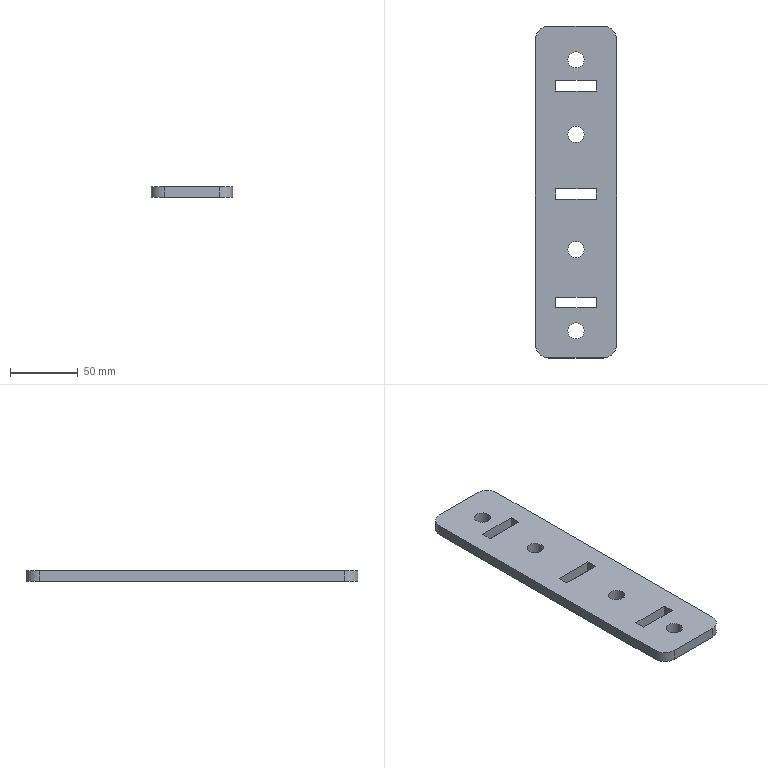Part | SolidWorks | features Fillet 1, FlatPattern 1, SMBaseFlange 1, SheetMetal 1 | 1 solid | 30 faces | box 60 x 245 x 8 mm | volume 107534 mm3 | plane 18 | cylinder 12 | commonest cylinder face diameters 12 x8 20 x4
STEP:
#1=CARTESIAN_POINT('',(-211.919,15.,8.));
#2=VERTEX_POINT('',#1);
#3=CARTESIAN_POINT('',(-199.919,15.,8.));
#4=VERTEX_POINT('',#3);
#5=CARTESIAN_POINT('',(-205.919,15.,8.));
#6=DIRECTION('',(0.,0.,1.));
#7=DIRECTION('',(1.,0.,0.));
#8=AXIS2_PLACEMENT_3D('',#5,#6,#7);
#9=CIRCLE('',#8,6.);
#10=EDGE_CURVE('',#2,#4,#9,.T.);
#11=ORIENTED_EDGE('',*,*,#10,.T.);
#12=CARTESIAN_POINT('',(-199.919,15.,0.));
#13=VERTEX_POINT('',#12);
#14=CARTESIAN_POINT('',(-199.919,15.,8.));
#15=DIRECTION('',(0.,0.,-1.));
#16=VECTOR('',#15,1000.);
#17=LINE('',#14,#16);
#18=EDGE_CURVE('',#4,#13,#17,.T.);
#19=ORIENTED_EDGE('',*,*,#18,.T.);
#20=CARTESIAN_POINT('',(-211.919,15.,0.));
#21=VERTEX_POINT('',#20);
#22=CARTESIAN_POINT('',(-205.919,15.,0.));
#23=DIRECTION('',(0.,0.,1.));
#24=DIRECTION('',(1.,0.,0.));
#25=AXIS2_PLACEMENT_3D('',#22,#23,#24);
#26=CIRCLE('',#25,6.);
#27=EDGE_CURVE('',#21,#13,#26,.T.);
#28=ORIENTED_EDGE('',*,*,#27,.F.);
#29=CARTESIAN_POINT('',(-211.919,15.,8.));
#30=DIRECTION('',(0.,0.,-1.));
#31=VECTOR('',#30,1000.);
#32=LINE('',#29,#31);
#33=EDGE_CURVE('',#2,#21,#32,.T.);
#34=ORIENTED_EDGE('',*,*,#33,.F.);
#35=EDGE_LOOP('',(#11,#19,#28,#34));
#36=FACE_OUTER_BOUND('',#35,.T.);
#37=CARTESIAN_POINT('',(-205.919,15.,8.));
#38=DIRECTION('',(0.,0.,-1.));
#39=DIRECTION('',(-1.,0.,0.));
#40=AXIS2_PLACEMENT_3D('',#37,#38,#39);
#41=CYLINDRICAL_SURFACE('',#40,6.);
#42=ADVANCED_FACE('',(#36),#41,.F.);
#43=CARTESIAN_POINT('',(-211.919,-185.,8.));
#44=VERTEX_POINT('',#43);
#45=CARTESIAN_POINT('',(-199.919,-185.,8.));
#46=VERTEX_POINT('',#45);
#47=CARTESIAN_POINT('',(-205.919,-185.,8.));
#48=DIRECTION('',(0.,0.,1.));
#49=DIRECTION('',(1.,0.,0.));
#50=AXIS2_PLACEMENT_3D('',#47,#48,#49);
#51=CIRCLE('',#50,6.);
#52=EDGE_CURVE('',#44,#46,#51,.T.);
#53=ORIENTED_EDGE('',*,*,#52,.T.);
#54=CARTESIAN_POINT('',(-199.919,-185.,0.));
#55=VERTEX_POINT('',#54);
#56=CARTESIAN_POINT('',(-199.919,-185.,8.));
#57=DIRECTION('',(0.,0.,-1.));
#58=VECTOR('',#57,1000.);
#59=LINE('',#56,#58);
#60=EDGE_CURVE('',#46,#55,#59,.T.);
#61=ORIENTED_EDGE('',*,*,#60,.T.);
#62=CARTESIAN_POINT('',(-211.919,-185.,0.));
#63=VERTEX_POINT('',#62);
#64=CARTESIAN_POINT('',(-205.919,-185.,0.));
#65=DIRECTION('',(0.,0.,1.));
#66=DIRECTION('',(1.,0.,0.));
#67=AXIS2_PLACEMENT_3D('',#64,#65,#66);
#68=CIRCLE('',#67,6.);
#69=EDGE_CURVE('',#63,#55,#68,.T.);
#70=ORIENTED_EDGE('',*,*,#69,.F.);
#71=CARTESIAN_POINT('',(-211.919,-185.,8.));
#72=DIRECTION('',(0.,0.,-1.));
#73=VECTOR('',#72,1000.);
#74=LINE('',#71,#73);
#75=EDGE_CURVE('',#44,#63,#74,.T.);
#76=ORIENTED_EDGE('',*,*,#75,.F.);
#77=EDGE_LOOP('',(#53,#61,#70,#76));
#78=FACE_OUTER_BOUND('',#77,.T.);
#79=CARTESIAN_POINT('',(-205.919,-185.,8.));
#80=DIRECTION('',(0.,0.,-1.));
#81=DIRECTION('',(-1.,0.,0.));
#82=AXIS2_PLACEMENT_3D('',#79,#80,#81);
#83=CYLINDRICAL_SURFACE('',#82,6.);
#84=ADVANCED_FACE('',(#78),#83,.F.);
#85=CARTESIAN_POINT('',(-211.919,-125.,8.));
#86=VERTEX_POINT('',#85);
#87=CARTESIAN_POINT('',(-199.919,-125.,8.));
#88=VERTEX_POINT('',#87);
#89=CARTESIAN_POINT('',(-205.919,-125.,8.));
#90=DIRECTION('',(0.,0.,1.));
#91=DIRECTION('',(1.,0.,0.));
#92=AXIS2_PLACEMENT_3D('',#89,#90,#91);
#93=CIRCLE('',#92,6.);
#94=EDGE_CURVE('',#86,#88,#93,.T.);
#95=ORIENTED_EDGE('',*,*,#94,.T.);
#96=CARTESIAN_POINT('',(-199.919,-125.,0.));
#97=VERTEX_POINT('',#96);
#98=CARTESIAN_POINT('',(-199.919,-125.,8.));
#99=DIRECTION('',(0.,0.,-1.));
#100=VECTOR('',#99,1000.);
#101=LINE('',#98,#100);
#102=EDGE_CURVE('',#88,#97,#101,.T.);
#103=ORIENTED_EDGE('',*,*,#102,.T.);
#104=CARTESIAN_POINT('',(-211.919,-125.,0.));
#105=VERTEX_POINT('',#104);
#106=CARTESIAN_POINT('',(-205.919,-125.,0.));
#107=DIRECTION('',(0.,0.,1.));
#108=DIRECTION('',(1.,0.,0.));
#109=AXIS2_PLACEMENT_3D('',#106,#107,#108);
#110=CIRCLE('',#109,6.);
#111=EDGE_CURVE('',#105,#97,#110,.T.);
#112=ORIENTED_EDGE('',*,*,#111,.F.);
#113=CARTESIAN_POINT('',(-211.919,-125.,8.));
#114=DIRECTION('',(0.,0.,-1.));
#115=VECTOR('',#114,1000.);
#116=LINE('',#113,#115);
#117=EDGE_CURVE('',#86,#105,#116,.T.);
#118=ORIENTED_EDGE('',*,*,#117,.F.);
#119=EDGE_LOOP('',(#95,#103,#112,#118));
#120=FACE_OUTER_BOUND('',#119,.T.);
#121=CARTESIAN_POINT('',(-205.919,-125.,8.));
#122=DIRECTION('',(0.,0.,-1.));
#123=DIRECTION('',(-1.,0.,0.));
#124=AXIS2_PLACEMENT_3D('',#121,#122,#123);
#125=CYLINDRICAL_SURFACE('',#124,6.);
#126=ADVANCED_FACE('',(#120),#125,.F.);
#127=CARTESIAN_POINT('',(-211.919,-40.,8.));
#128=VERTEX_POINT('',#127);
#129=CARTESIAN_POINT('',(-199.919,-40.,8.));
#130=VERTEX_POINT('',#129);
#131=CARTESIAN_POINT('',(-205.919,-40.,8.));
#132=DIRECTION('',(0.,0.,1.));
#133=DIRECTION('',(1.,0.,0.));
#134=AXIS2_PLACEMENT_3D('',#131,#132,#133);
#135=CIRCLE('',#134,6.);
#136=EDGE_CURVE('',#128,#130,#135,.T.);
#137=ORIENTED_EDGE('',*,*,#136,.T.);
#138=CARTESIAN_POINT('',(-199.919,-40.,0.));
#139=VERTEX_POINT('',#138);
#140=CARTESIAN_POINT('',(-199.919,-40.,8.));
#141=DIRECTION('',(0.,0.,-1.));
#142=VECTOR('',#141,1000.);
#143=LINE('',#140,#142);
#144=EDGE_CURVE('',#130,#139,#143,.T.);
#145=ORIENTED_EDGE('',*,*,#144,.T.);
#146=CARTESIAN_POINT('',(-211.919,-40.,0.));
#147=VERTEX_POINT('',#146);
#148=CARTESIAN_POINT('',(-205.919,-40.,0.));
#149=DIRECTION('',(0.,0.,1.));
#150=DIRECTION('',(1.,0.,0.));
#151=AXIS2_PLACEMENT_3D('',#148,#149,#150);
#152=CIRCLE('',#151,6.);
#153=EDGE_CURVE('',#147,#139,#152,.T.);
#154=ORIENTED_EDGE('',*,*,#153,.F.);
#155=CARTESIAN_POINT('',(-211.919,-40.,8.));
#156=DIRECTION('',(0.,0.,-1.));
#157=VECTOR('',#156,1000.);
#158=LINE('',#155,#157);
#159=EDGE_CURVE('',#128,#147,#158,.T.);
#160=ORIENTED_EDGE('',*,*,#159,.F.);
#161=EDGE_LOOP('',(#137,#145,#154,#160));
#162=FACE_OUTER_BOUND('',#161,.T.);
#163=CARTESIAN_POINT('',(-205.919,-40.,8.));
#164=DIRECTION('',(0.,0.,-1.));
#165=DIRECTION('',(-1.,0.,0.));
#166=AXIS2_PLACEMENT_3D('',#163,#164,#165);
#167=CYLINDRICAL_SURFACE('',#166,6.);
#168=ADVANCED_FACE('',(#162),#167,.F.);
#169=ORIENTED_EDGE('',*,*,#52,.F.);
#170=CARTESIAN_POINT('',(-205.919,-185.,8.));
#171=DIRECTION('',(0.,0.,1.));
#172=DIRECTION('',(1.,0.,0.));
#173=AXIS2_PLACEMENT_3D('',#170,#171,#172);
#174=CIRCLE('',#173,6.);
#175=EDGE_CURVE('',#46,#44,#174,.T.);
#176=ORIENTED_EDGE('',*,*,#175,.F.);
#177=EDGE_LOOP('',(#169,#176));
#178=FACE_BOUND('',#177,.T.);
#179=ORIENTED_EDGE('',*,*,#136,.F.);
#180=CARTESIAN_POINT('',(-205.919,-40.,8.));
#181=DIRECTION('',(0.,0.,1.));
#182=DIRECTION('',(1.,0.,0.));
#183=AXIS2_PLACEMENT_3D('',#180,#181,#182);
#184=CIRCLE('',#183,6.);
#185=EDGE_CURVE('',#130,#128,#184,.T.);
#186=ORIENTED_EDGE('',*,*,#185,.F.);
#187=EDGE_LOOP('',(#179,#186));
#188=FACE_BOUND('',#187,.T.);
#189=CARTESIAN_POINT('',(-235.919,30.,8.));
#190=VERTEX_POINT('',#189);
#191=CARTESIAN_POINT('',(-235.919,-195.,8.));
#192=VERTEX_POINT('',#191);
#193=CARTESIAN_POINT('',(-235.919,40.,8.));
#194=DIRECTION('',(0.,-1.,0.));
#195=VECTOR('',#194,1000.);
#196=LINE('',#193,#195);
#197=EDGE_CURVE('',#190,#192,#196,.T.);
#198=ORIENTED_EDGE('',*,*,#197,.T.);
#199=CARTESIAN_POINT('',(-225.919,-205.,8.));
#200=VERTEX_POINT('',#199);
#201=CARTESIAN_POINT('',(-225.919,-195.,8.));
#202=DIRECTION('',(0.,0.,1.));
#203=DIRECTION('',(1.,0.,0.));
#204=AXIS2_PLACEMENT_3D('',#201,#202,#203);
#205=CIRCLE('',#204,10.);
#206=EDGE_CURVE('',#192,#200,#205,.T.);
#207=ORIENTED_EDGE('',*,*,#206,.T.);
#208=CARTESIAN_POINT('',(-185.919,-205.,8.));
#209=VERTEX_POINT('',#208);
#210=CARTESIAN_POINT('',(-235.919,-205.,8.));
#211=DIRECTION('',(1.,0.,0.));
#212=VECTOR('',#211,1000.);
#213=LINE('',#210,#212);
#214=EDGE_CURVE('',#200,#209,#213,.T.);
#215=ORIENTED_EDGE('',*,*,#214,.T.);
#216=CARTESIAN_POINT('',(-175.919,-195.,8.));
#217=VERTEX_POINT('',#216);
#218=CARTESIAN_POINT('',(-185.919,-195.,8.));
#219=DIRECTION('',(0.,0.,1.));
#220=DIRECTION('',(1.,0.,0.));
#221=AXIS2_PLACEMENT_3D('',#218,#219,#220);
#222=CIRCLE('',#221,10.);
#223=EDGE_CURVE('',#209,#217,#222,.T.);
#224=ORIENTED_EDGE('',*,*,#223,.T.);
#225=CARTESIAN_POINT('',(-175.919,30.,8.));
#226=VERTEX_POINT('',#225);
#227=CARTESIAN_POINT('',(-175.919,-205.,8.));
#228=DIRECTION('',(0.,1.,0.));
#229=VECTOR('',#228,1000.);
#230=LINE('',#227,#229);
#231=EDGE_CURVE('',#217,#226,#230,.T.);
#232=ORIENTED_EDGE('',*,*,#231,.T.);
#233=CARTESIAN_POINT('',(-185.919,40.,8.));
#234=VERTEX_POINT('',#233);
#235=CARTESIAN_POINT('',(-185.919,30.,8.));
#236=DIRECTION('',(0.,0.,1.));
#237=DIRECTION('',(1.,0.,0.));
#238=AXIS2_PLACEMENT_3D('',#235,#236,#237);
#239=CIRCLE('',#238,10.);
#240=EDGE_CURVE('',#226,#234,#239,.T.);
#241=ORIENTED_EDGE('',*,*,#240,.T.);
#242=CARTESIAN_POINT('',(-225.919,40.,8.));
#243=VERTEX_POINT('',#242);
#244=CARTESIAN_POINT('',(-175.919,40.,8.));
#245=DIRECTION('',(-1.,0.,0.));
#246=VECTOR('',#245,1000.);
#247=LINE('',#244,#246);
#248=EDGE_CURVE('',#234,#243,#247,.T.);
#249=ORIENTED_EDGE('',*,*,#248,.T.);
#250=CARTESIAN_POINT('',(-225.919,30.,8.));
#251=DIRECTION('',(0.,0.,1.));
#252=DIRECTION('',(1.,0.,0.));
#253=AXIS2_PLACEMENT_3D('',#250,#251,#252);
#254=CIRCLE('',#253,10.);
#255=EDGE_CURVE('',#243,#190,#254,.T.);
#256=ORIENTED_EDGE('',*,*,#255,.T.);
#257=EDGE_LOOP('',(#198,#207,#215,#224,#232,#241,#249,#256));
#258=FACE_OUTER_BOUND('',#257,.T.);
#259=CARTESIAN_POINT('',(-190.919,-160.,8.));
#260=VERTEX_POINT('',#259);
#261=CARTESIAN_POINT('',(-220.919,-160.,8.));
#262=VERTEX_POINT('',#261);
#263=CARTESIAN_POINT('',(-220.919,-160.,8.));
#264=DIRECTION('',(-1.,0.,0.));
#265=VECTOR('',#264,1000.);
#266=LINE('',#263,#265);
#267=EDGE_CURVE('',#260,#262,#266,.T.);
#268=ORIENTED_EDGE('',*,*,#267,.F.);
#269=CARTESIAN_POINT('',(-190.919,-168.,8.));
#270=VERTEX_POINT('',#269);
#271=CARTESIAN_POINT('',(-190.919,-160.,8.));
#272=DIRECTION('',(0.,1.,0.));
#273=VECTOR('',#272,1000.);
#274=LINE('',#271,#273);
#275=EDGE_CURVE('',#270,#260,#274,.T.);
#276=ORIENTED_EDGE('',*,*,#275,.F.);
#277=CARTESIAN_POINT('',(-220.919,-168.,8.));
#278=VERTEX_POINT('',#277);
#279=CARTESIAN_POINT('',(-190.919,-168.,8.));
#280=DIRECTION('',(1.,0.,0.));
#281=VECTOR('',#280,1000.);
#282=LINE('',#279,#281);
#283=EDGE_CURVE('',#278,#270,#282,.T.);
#284=ORIENTED_EDGE('',*,*,#283,.F.);
#285=CARTESIAN_POINT('',(-220.919,-168.,8.));
#286=DIRECTION('',(0.,-1.,0.));
#287=VECTOR('',#286,1000.);
#288=LINE('',#285,#287);
#289=EDGE_CURVE('',#262,#278,#288,.T.);
#290=ORIENTED_EDGE('',*,*,#289,.F.);
#291=EDGE_LOOP('',(#268,#276,#284,#290));
#292=FACE_BOUND('',#291,.T.);
#293=CARTESIAN_POINT('',(-190.919,-88.,8.));
#294=VERTEX_POINT('',#293);
#295=CARTESIAN_POINT('',(-190.919,-80.,8.));
#296=VERTEX_POINT('',#295);
#297=CARTESIAN_POINT('',(-190.919,-80.,8.));
#298=DIRECTION('',(0.,1.,0.));
#299=VECTOR('',#298,1000.);
#300=LINE('',#297,#299);
#301=EDGE_CURVE('',#294,#296,#300,.T.);
#302=ORIENTED_EDGE('',*,*,#301,.F.);
#303=CARTESIAN_POINT('',(-220.919,-88.,8.));
#304=VERTEX_POINT('',#303);
#305=CARTESIAN_POINT('',(-190.919,-88.,8.));
#306=DIRECTION('',(1.,0.,0.));
#307=VECTOR('',#306,1000.);
#308=LINE('',#305,#307);
#309=EDGE_CURVE('',#304,#294,#308,.T.);
#310=ORIENTED_EDGE('',*,*,#309,.F.);
#311=CARTESIAN_POINT('',(-220.919,-80.,8.));
#312=VERTEX_POINT('',#311);
#313=CARTESIAN_POINT('',(-220.919,-88.,8.));
#314=DIRECTION('',(0.,-1.,0.));
#315=VECTOR('',#314,1000.);
#316=LINE('',#313,#315);
#317=EDGE_CURVE('',#312,#304,#316,.T.);
#318=ORIENTED_EDGE('',*,*,#317,.F.);
#319=CARTESIAN_POINT('',(-220.919,-80.,8.));
#320=DIRECTION('',(-1.,0.,0.));
#321=VECTOR('',#320,1000.);
#322=LINE('',#319,#321);
#323=EDGE_CURVE('',#296,#312,#322,.T.);
#324=ORIENTED_EDGE('',*,*,#323,.F.);
#325=EDGE_LOOP('',(#302,#310,#318,#324));
#326=FACE_BOUND('',#325,.T.);
#327=CARTESIAN_POINT('',(-190.919,-8.,8.));
#328=VERTEX_POINT('',#327);
#329=CARTESIAN_POINT('',(-190.919,0.,8.));
#330=VERTEX_POINT('',#329);
#331=CARTESIAN_POINT('',(-190.919,0.,8.));
#332=DIRECTION('',(0.,1.,0.));
#333=VECTOR('',#332,1000.);
#334=LINE('',#331,#333);
#335=EDGE_CURVE('',#328,#330,#334,.T.);
#336=ORIENTED_EDGE('',*,*,#335,.F.);
#337=CARTESIAN_POINT('',(-220.919,-8.,8.));
#338=VERTEX_POINT('',#337);
#339=CARTESIAN_POINT('',(-190.919,-8.,8.));
#340=DIRECTION('',(1.,0.,0.));
#341=VECTOR('',#340,1000.);
#342=LINE('',#339,#341);
#343=EDGE_CURVE('',#338,#328,#342,.T.);
#344=ORIENTED_EDGE('',*,*,#343,.F.);
#345=CARTESIAN_POINT('',(-220.919,0.,8.));
#346=VERTEX_POINT('',#345);
#347=CARTESIAN_POINT('',(-220.919,-8.,8.));
#348=DIRECTION('',(0.,-1.,0.));
#349=VECTOR('',#348,1000.);
#350=LINE('',#347,#349);
#351=EDGE_CURVE('',#346,#338,#350,.T.);
#352=ORIENTED_EDGE('',*,*,#351,.F.);
#353=CARTESIAN_POINT('',(-220.919,0.,8.));
#354=DIRECTION('',(-1.,0.,0.));
#355=VECTOR('',#354,1000.);
#356=LINE('',#353,#355);
#357=EDGE_CURVE('',#330,#346,#356,.T.);
#358=ORIENTED_EDGE('',*,*,#357,.F.);
#359=EDGE_LOOP('',(#336,#344,#352,#358));
#360=FACE_BOUND('',#359,.T.);
#361=ORIENTED_EDGE('',*,*,#94,.F.);
#362=CARTESIAN_POINT('',(-205.919,-125.,8.));
#363=DIRECTION('',(0.,0.,1.));
#364=DIRECTION('',(1.,0.,0.));
#365=AXIS2_PLACEMENT_3D('',#362,#363,#364);
#366=CIRCLE('',#365,6.);
#367=EDGE_CURVE('',#88,#86,#366,.T.);
#368=ORIENTED_EDGE('',*,*,#367,.F.);
#369=EDGE_LOOP('',(#361,#368));
#370=FACE_BOUND('',#369,.T.);
#371=ORIENTED_EDGE('',*,*,#10,.F.);
#372=CARTESIAN_POINT('',(-205.919,15.,8.));
#373=DIRECTION('',(0.,0.,1.));
#374=DIRECTION('',(1.,0.,0.));
#375=AXIS2_PLACEMENT_3D('',#372,#373,#374);
#376=CIRCLE('',#375,6.);
#377=EDGE_CURVE('',#4,#2,#376,.T.);
#378=ORIENTED_EDGE('',*,*,#377,.F.);
#379=EDGE_LOOP('',(#371,#378));
#380=FACE_BOUND('',#379,.T.);
#381=CARTESIAN_POINT('',(0.,0.,8.));
#382=DIRECTION('',(0.,0.,1.));
#383=DIRECTION('',(1.,0.,0.));
#384=AXIS2_PLACEMENT_3D('',#381,#382,#383);
#385=PLANE('',#384);
#386=ADVANCED_FACE('',(#178,#188,#258,#292,#326,#360,#370,#380),#385,.T.);
#387=CARTESIAN_POINT('',(-220.919,-88.,0.));
#388=VERTEX_POINT('',#387);
#389=CARTESIAN_POINT('',(-190.919,-88.,0.));
#390=VERTEX_POINT('',#389);
#391=CARTESIAN_POINT('',(-190.919,-88.,0.));
#392=DIRECTION('',(1.,0.,0.));
#393=VECTOR('',#392,1000.);
#394=LINE('',#391,#393);
#395=EDGE_CURVE('',#388,#390,#394,.T.);
#396=ORIENTED_EDGE('',*,*,#395,.T.);
#397=CARTESIAN_POINT('',(-190.919,-80.,0.));
#398=VERTEX_POINT('',#397);
#399=CARTESIAN_POINT('',(-190.919,-80.,0.));
#400=DIRECTION('',(0.,1.,0.));
#401=VECTOR('',#400,1000.);
#402=LINE('',#399,#401);
#403=EDGE_CURVE('',#390,#398,#402,.T.);
#404=ORIENTED_EDGE('',*,*,#403,.T.);
#405=CARTESIAN_POINT('',(-220.919,-80.,0.));
#406=VERTEX_POINT('',#405);
#407=CARTESIAN_POINT('',(-220.919,-80.,0.));
#408=DIRECTION('',(-1.,0.,0.));
#409=VECTOR('',#408,1000.);
#410=LINE('',#407,#409);
#411=EDGE_CURVE('',#398,#406,#410,.T.);
#412=ORIENTED_EDGE('',*,*,#411,.T.);
#413=CARTESIAN_POINT('',(-220.919,-88.,0.));
#414=DIRECTION('',(0.,-1.,0.));
#415=VECTOR('',#414,1000.);
#416=LINE('',#413,#415);
#417=EDGE_CURVE('',#406,#388,#416,.T.);
#418=ORIENTED_EDGE('',*,*,#417,.T.);
#419=EDGE_LOOP('',(#396,#404,#412,#418));
#420=FACE_BOUND('',#419,.T.);
#421=CARTESIAN_POINT('',(-225.919,-205.,0.));
#422=VERTEX_POINT('',#421);
#423=CARTESIAN_POINT('',(-185.919,-205.,0.));
#424=VERTEX_POINT('',#423);
#425=CARTESIAN_POINT('',(-235.919,-205.,0.));
#426=DIRECTION('',(1.,0.,0.));
#427=VECTOR('',#426,1000.);
#428=LINE('',#425,#427);
#429=EDGE_CURVE('',#422,#424,#428,.T.);
#430=ORIENTED_EDGE('',*,*,#429,.F.);
#431=CARTESIAN_POINT('',(-235.919,-195.,0.));
#432=VERTEX_POINT('',#431);
#433=CARTESIAN_POINT('',(-225.919,-195.,0.));
#434=DIRECTION('',(0.,0.,-1.));
#435=DIRECTION('',(1.,0.,0.));
#436=AXIS2_PLACEMENT_3D('',#433,#434,#435);
#437=CIRCLE('',#436,10.);
#438=EDGE_CURVE('',#422,#432,#437,.T.);
#439=ORIENTED_EDGE('',*,*,#438,.T.);
#440=CARTESIAN_POINT('',(-235.919,30.,0.));
#441=VERTEX_POINT('',#440);
#442=CARTESIAN_POINT('',(-235.919,40.,0.));
#443=DIRECTION('',(0.,-1.,0.));
#444=VECTOR('',#443,1000.);
#445=LINE('',#442,#444);
#446=EDGE_CURVE('',#441,#432,#445,.T.);
#447=ORIENTED_EDGE('',*,*,#446,.F.);
#448=CARTESIAN_POINT('',(-225.919,40.,0.));
#449=VERTEX_POINT('',#448);
#450=CARTESIAN_POINT('',(-225.919,30.,0.));
#451=DIRECTION('',(0.,0.,-1.));
#452=DIRECTION('',(1.,0.,0.));
#453=AXIS2_PLACEMENT_3D('',#450,#451,#452);
#454=CIRCLE('',#453,10.);
#455=EDGE_CURVE('',#441,#449,#454,.T.);
#456=ORIENTED_EDGE('',*,*,#455,.T.);
#457=CARTESIAN_POINT('',(-185.919,40.,0.));
#458=VERTEX_POINT('',#457);
#459=CARTESIAN_POINT('',(-175.919,40.,0.));
#460=DIRECTION('',(-1.,0.,0.));
#461=VECTOR('',#460,1000.);
#462=LINE('',#459,#461);
#463=EDGE_CURVE('',#458,#449,#462,.T.);
#464=ORIENTED_EDGE('',*,*,#463,.F.);
#465=CARTESIAN_POINT('',(-175.919,30.,0.));
#466=VERTEX_POINT('',#465);
#467=CARTESIAN_POINT('',(-185.919,30.,0.));
#468=DIRECTION('',(0.,0.,-1.));
#469=DIRECTION('',(1.,0.,0.));
#470=AXIS2_PLACEMENT_3D('',#467,#468,#469);
#471=CIRCLE('',#470,10.);
#472=EDGE_CURVE('',#458,#466,#471,.T.);
#473=ORIENTED_EDGE('',*,*,#472,.T.);
#474=CARTESIAN_POINT('',(-175.919,-195.,0.));
#475=VERTEX_POINT('',#474);
#476=CARTESIAN_POINT('',(-175.919,-205.,0.));
#477=DIRECTION('',(0.,1.,0.));
#478=VECTOR('',#477,1000.);
#479=LINE('',#476,#478);
#480=EDGE_CURVE('',#475,#466,#479,.T.);
#481=ORIENTED_EDGE('',*,*,#480,.F.);
#482=CARTESIAN_POINT('',(-185.919,-195.,0.));
#483=DIRECTION('',(0.,0.,-1.));
#484=DIRECTION('',(1.,0.,0.));
#485=AXIS2_PLACEMENT_3D('',#482,#483,#484);
#486=CIRCLE('',#485,10.);
#487=EDGE_CURVE('',#475,#424,#486,.T.);
#488=ORIENTED_EDGE('',*,*,#487,.T.);
#489=EDGE_LOOP('',(#430,#439,#447,#456,#464,#473,#481,#488));
#490=FACE_OUTER_BOUND('',#489,.T.);
#491=CARTESIAN_POINT('',(-190.919,-168.,0.));
#492=VERTEX_POINT('',#491);
#493=CARTESIAN_POINT('',(-190.919,-160.,0.));
#494=VERTEX_POINT('',#493);
#495=CARTESIAN_POINT('',(-190.919,-160.,0.));
#496=DIRECTION('',(0.,1.,0.));
#497=VECTOR('',#496,1000.);
#498=LINE('',#495,#497);
#499=EDGE_CURVE('',#492,#494,#498,.T.);
#500=ORIENTED_EDGE('',*,*,#499,.T.);
#501=CARTESIAN_POINT('',(-220.919,-160.,0.));
#502=VERTEX_POINT('',#501);
#503=CARTESIAN_POINT('',(-220.919,-160.,0.));
#504=DIRECTION('',(-1.,0.,0.));
#505=VECTOR('',#504,1000.);
#506=LINE('',#503,#505);
#507=EDGE_CURVE('',#494,#502,#506,.T.);
#508=ORIENTED_EDGE('',*,*,#507,.T.);
#509=CARTESIAN_POINT('',(-220.919,-168.,0.));
#510=VERTEX_POINT('',#509);
#511=CARTESIAN_POINT('',(-220.919,-168.,0.));
#512=DIRECTION('',(0.,-1.,0.));
#513=VECTOR('',#512,1000.);
#514=LINE('',#511,#513);
#515=EDGE_CURVE('',#502,#510,#514,.T.);
#516=ORIENTED_EDGE('',*,*,#515,.T.);
#517=CARTESIAN_POINT('',(-190.919,-168.,0.));
#518=DIRECTION('',(1.,0.,0.));
#519=VECTOR('',#518,1000.);
#520=LINE('',#517,#519);
#521=EDGE_CURVE('',#510,#492,#520,.T.);
#522=ORIENTED_EDGE('',*,*,#521,.T.);
#523=EDGE_LOOP('',(#500,#508,#516,#522));
#524=FACE_BOUND('',#523,.T.);
#525=CARTESIAN_POINT('',(-220.919,-8.,0.));
#526=VERTEX_POINT('',#525);
#527=CARTESIAN_POINT('',(-190.919,-8.,0.));
#528=VERTEX_POINT('',#527);
#529=CARTESIAN_POINT('',(-190.919,-8.,0.));
#530=DIRECTION('',(1.,0.,0.));
#531=VECTOR('',#530,1000.);
#532=LINE('',#529,#531);
#533=EDGE_CURVE('',#526,#528,#532,.T.);
#534=ORIENTED_EDGE('',*,*,#533,.T.);
#535=CARTESIAN_POINT('',(-190.919,0.,0.));
#536=VERTEX_POINT('',#535);
#537=CARTESIAN_POINT('',(-190.919,0.,0.));
#538=DIRECTION('',(0.,1.,0.));
#539=VECTOR('',#538,1000.);
#540=LINE('',#537,#539);
#541=EDGE_CURVE('',#528,#536,#540,.T.);
#542=ORIENTED_EDGE('',*,*,#541,.T.);
#543=CARTESIAN_POINT('',(-220.919,0.,0.));
#544=VERTEX_POINT('',#543);
#545=CARTESIAN_POINT('',(-220.919,0.,0.));
#546=DIRECTION('',(-1.,0.,0.));
#547=VECTOR('',#546,1000.);
#548=LINE('',#545,#547);
#549=EDGE_CURVE('',#536,#544,#548,.T.);
#550=ORIENTED_EDGE('',*,*,#549,.T.);
#551=CARTESIAN_POINT('',(-220.919,-8.,0.));
#552=DIRECTION('',(0.,-1.,0.));
#553=VECTOR('',#552,1000.);
#554=LINE('',#551,#553);
#555=EDGE_CURVE('',#544,#526,#554,.T.);
#556=ORIENTED_EDGE('',*,*,#555,.T.);
#557=EDGE_LOOP('',(#534,#542,#550,#556));
#558=FACE_BOUND('',#557,.T.);
#559=ORIENTED_EDGE('',*,*,#153,.T.);
#560=CARTESIAN_POINT('',(-205.919,-40.,0.));
#561=DIRECTION('',(0.,0.,1.));
#562=DIRECTION('',(1.,0.,0.));
#563=AXIS2_PLACEMENT_3D('',#560,#561,#562);
#564=CIRCLE('',#563,6.);
#565=EDGE_CURVE('',#139,#147,#564,.T.);
#566=ORIENTED_EDGE('',*,*,#565,.T.);
#567=EDGE_LOOP('',(#559,#566));
#568=FACE_BOUND('',#567,.T.);
#569=ORIENTED_EDGE('',*,*,#111,.T.);
#570=CARTESIAN_POINT('',(-205.919,-125.,0.));
#571=DIRECTION('',(0.,0.,1.));
#572=DIRECTION('',(1.,0.,0.));
#573=AXIS2_PLACEMENT_3D('',#570,#571,#572);
#574=CIRCLE('',#573,6.);
#575=EDGE_CURVE('',#97,#105,#574,.T.);
#576=ORIENTED_EDGE('',*,*,#575,.T.);
#577=EDGE_LOOP('',(#569,#576));
#578=FACE_BOUND('',#577,.T.);
#579=ORIENTED_EDGE('',*,*,#69,.T.);
#580=CARTESIAN_POINT('',(-205.919,-185.,0.));
#581=DIRECTION('',(0.,0.,1.));
#582=DIRECTION('',(1.,0.,0.));
#583=AXIS2_PLACEMENT_3D('',#580,#581,#582);
#584=CIRCLE('',#583,6.);
#585=EDGE_CURVE('',#55,#63,#584,.T.);
#586=ORIENTED_EDGE('',*,*,#585,.T.);
#587=EDGE_LOOP('',(#579,#586));
#588=FACE_BOUND('',#587,.T.);
#589=ORIENTED_EDGE('',*,*,#27,.T.);
#590=CARTESIAN_POINT('',(-205.919,15.,0.));
#591=DIRECTION('',(0.,0.,1.));
#592=DIRECTION('',(1.,0.,0.));
#593=AXIS2_PLACEMENT_3D('',#590,#591,#592);
#594=CIRCLE('',#593,6.);
#595=EDGE_CURVE('',#13,#21,#594,.T.);
#596=ORIENTED_EDGE('',*,*,#595,.T.);
#597=EDGE_LOOP('',(#589,#596));
#598=FACE_BOUND('',#597,.T.);
#599=CARTESIAN_POINT('',(0.,0.,0.));
#600=DIRECTION('',(0.,0.,1.));
#601=DIRECTION('',(1.,0.,0.));
#602=AXIS2_PLACEMENT_3D('',#599,#600,#601);
#603=PLANE('',#602);
#604=ADVANCED_FACE('',(#420,#490,#524,#558,#568,#578,#588,#598),#603,.F.);
#605=ORIENTED_EDGE('',*,*,#446,.T.);
#606=CARTESIAN_POINT('',(-235.919,-195.,8.));
#607=DIRECTION('',(0.,0.,1.));
#608=VECTOR('',#607,1000.);
#609=LINE('',#606,#608);
#610=EDGE_CURVE('',#432,#192,#609,.T.);
#611=ORIENTED_EDGE('',*,*,#610,.T.);
#612=ORIENTED_EDGE('',*,*,#197,.F.);
#613=CARTESIAN_POINT('',(-235.919,30.,8.));
#614=DIRECTION('',(0.,0.,-1.));
#615=VECTOR('',#614,1000.);
#616=LINE('',#613,#615);
#617=EDGE_CURVE('',#190,#441,#616,.T.);
#618=ORIENTED_EDGE('',*,*,#617,.T.);
#619=EDGE_LOOP('',(#605,#611,#612,#618));
#620=FACE_OUTER_BOUND('',#619,.T.);
#621=CARTESIAN_POINT('',(-235.919,40.,8.));
#622=DIRECTION('',(1.,0.,0.));
#623=DIRECTION('',(0.,1.,0.));
#624=AXIS2_PLACEMENT_3D('',#621,#622,#623);
#625=PLANE('',#624);
#626=ADVANCED_FACE('',(#620),#625,.F.);
#627=ORIENTED_EDGE('',*,*,#214,.F.);
#628=CARTESIAN_POINT('',(-225.919,-205.,8.));
#629=DIRECTION('',(0.,0.,-1.));
#630=VECTOR('',#629,1000.);
#631=LINE('',#628,#630);
#632=EDGE_CURVE('',#200,#422,#631,.T.);
#633=ORIENTED_EDGE('',*,*,#632,.T.);
#634=ORIENTED_EDGE('',*,*,#429,.T.);
#635=CARTESIAN_POINT('',(-185.919,-205.,8.));
#636=DIRECTION('',(0.,0.,1.));
#637=VECTOR('',#636,1000.);
#638=LINE('',#635,#637);
#639=EDGE_CURVE('',#424,#209,#638,.T.);
#640=ORIENTED_EDGE('',*,*,#639,.T.);
#641=EDGE_LOOP('',(#627,#633,#634,#640));
#642=FACE_OUTER_BOUND('',#641,.T.);
#643=CARTESIAN_POINT('',(-235.919,-205.,8.));
#644=DIRECTION('',(0.,1.,0.));
#645=DIRECTION('',(0.,0.,1.));
#646=AXIS2_PLACEMENT_3D('',#643,#644,#645);
#647=PLANE('',#646);
#648=ADVANCED_FACE('',(#642),#647,.F.);
#649=ORIENTED_EDGE('',*,*,#231,.F.);
#650=CARTESIAN_POINT('',(-175.919,-195.,8.));
#651=DIRECTION('',(0.,0.,-1.));
#652=VECTOR('',#651,1000.);
#653=LINE('',#650,#652);
#654=EDGE_CURVE('',#217,#475,#653,.T.);
#655=ORIENTED_EDGE('',*,*,#654,.T.);
#656=ORIENTED_EDGE('',*,*,#480,.T.);
#657=CARTESIAN_POINT('',(-175.919,30.,8.));
#658=DIRECTION('',(0.,0.,1.));
#659=VECTOR('',#658,1000.);
#660=LINE('',#657,#659);
#661=EDGE_CURVE('',#466,#226,#660,.T.);
#662=ORIENTED_EDGE('',*,*,#661,.T.);
#663=EDGE_LOOP('',(#649,#655,#656,#662));
#664=FACE_OUTER_BOUND('',#663,.T.);
#665=CARTESIAN_POINT('',(-175.919,-205.,8.));
#666=DIRECTION('',(-1.,0.,0.));
#667=DIRECTION('',(0.,0.,1.));
#668=AXIS2_PLACEMENT_3D('',#665,#666,#667);
#669=PLANE('',#668);
#670=ADVANCED_FACE('',(#664),#669,.F.);
#671=ORIENTED_EDGE('',*,*,#248,.F.);
#672=CARTESIAN_POINT('',(-185.919,40.,8.));
#673=DIRECTION('',(0.,0.,-1.));
#674=VECTOR('',#673,1000.);
#675=LINE('',#672,#674);
#676=EDGE_CURVE('',#234,#458,#675,.T.);
#677=ORIENTED_EDGE('',*,*,#676,.T.);
#678=ORIENTED_EDGE('',*,*,#463,.T.);
#679=CARTESIAN_POINT('',(-225.919,40.,8.));
#680=DIRECTION('',(0.,0.,1.));
#681=VECTOR('',#680,1000.);
#682=LINE('',#679,#681);
#683=EDGE_CURVE('',#449,#243,#682,.T.);
#684=ORIENTED_EDGE('',*,*,#683,.T.);
#685=EDGE_LOOP('',(#671,#677,#678,#684));
#686=FACE_OUTER_BOUND('',#685,.T.);
#687=CARTESIAN_POINT('',(-175.919,40.,8.));
#688=DIRECTION('',(0.,-1.,0.));
#689=DIRECTION('',(1.,0.,0.));
#690=AXIS2_PLACEMENT_3D('',#687,#688,#689);
#691=PLANE('',#690);
#692=ADVANCED_FACE('',(#686),#691,.F.);
#693=ORIENTED_EDGE('',*,*,#499,.F.);
#694=CARTESIAN_POINT('',(-190.919,-168.,8.));
#695=DIRECTION('',(0.,0.,-1.));
#696=VECTOR('',#695,1000.);
#697=LINE('',#694,#696);
#698=EDGE_CURVE('',#270,#492,#697,.T.);
#699=ORIENTED_EDGE('',*,*,#698,.F.);
#700=ORIENTED_EDGE('',*,*,#275,.T.);
#701=CARTESIAN_POINT('',(-190.919,-160.,8.));
#702=DIRECTION('',(0.,0.,-1.));
#703=VECTOR('',#702,1000.);
#704=LINE('',#701,#703);
#705=EDGE_CURVE('',#260,#494,#704,.T.);
#706=ORIENTED_EDGE('',*,*,#705,.T.);
#707=EDGE_LOOP('',(#693,#699,#700,#706));
#708=FACE_OUTER_BOUND('',#707,.T.);
#709=CARTESIAN_POINT('',(-190.919,-160.,8.));
#710=DIRECTION('',(-1.,0.,0.));
#711=DIRECTION('',(0.,0.,1.));
#712=AXIS2_PLACEMENT_3D('',#709,#710,#711);
#713=PLANE('',#712);
#714=ADVANCED_FACE('',(#708),#713,.T.);
#715=ORIENTED_EDGE('',*,*,#507,.F.);
#716=ORIENTED_EDGE('',*,*,#705,.F.);
#717=ORIENTED_EDGE('',*,*,#267,.T.);
#718=CARTESIAN_POINT('',(-220.919,-160.,8.));
#719=DIRECTION('',(0.,0.,-1.));
#720=VECTOR('',#719,1000.);
#721=LINE('',#718,#720);
#722=EDGE_CURVE('',#262,#502,#721,.T.);
#723=ORIENTED_EDGE('',*,*,#722,.T.);
#724=EDGE_LOOP('',(#715,#716,#717,#723));
#725=FACE_OUTER_BOUND('',#724,.T.);
#726=CARTESIAN_POINT('',(-220.919,-160.,8.));
#727=DIRECTION('',(0.,-1.,0.));
#728=DIRECTION('',(0.,0.,-1.));
#729=AXIS2_PLACEMENT_3D('',#726,#727,#728);
#730=PLANE('',#729);
#731=ADVANCED_FACE('',(#725),#730,.T.);
#732=ORIENTED_EDGE('',*,*,#515,.F.);
#733=ORIENTED_EDGE('',*,*,#722,.F.);
#734=ORIENTED_EDGE('',*,*,#289,.T.);
#735=CARTESIAN_POINT('',(-220.919,-168.,8.));
#736=DIRECTION('',(0.,0.,-1.));
#737=VECTOR('',#736,1000.);
#738=LINE('',#735,#737);
#739=EDGE_CURVE('',#278,#510,#738,.T.);
#740=ORIENTED_EDGE('',*,*,#739,.T.);
#741=EDGE_LOOP('',(#732,#733,#734,#740));
#742=FACE_OUTER_BOUND('',#741,.T.);
#743=CARTESIAN_POINT('',(-220.919,-168.,8.));
#744=DIRECTION('',(1.,0.,0.));
#745=DIRECTION('',(0.,0.,-1.));
#746=AXIS2_PLACEMENT_3D('',#743,#744,#745);
#747=PLANE('',#746);
#748=ADVANCED_FACE('',(#742),#747,.T.);
#749=ORIENTED_EDGE('',*,*,#521,.F.);
#750=ORIENTED_EDGE('',*,*,#739,.F.);
#751=ORIENTED_EDGE('',*,*,#283,.T.);
#752=ORIENTED_EDGE('',*,*,#698,.T.);
#753=EDGE_LOOP('',(#749,#750,#751,#752));
#754=FACE_OUTER_BOUND('',#753,.T.);
#755=CARTESIAN_POINT('',(-190.919,-168.,8.));
#756=DIRECTION('',(0.,1.,0.));
#757=DIRECTION('',(0.,0.,1.));
#758=AXIS2_PLACEMENT_3D('',#755,#756,#757);
#759=PLANE('',#758);
#760=ADVANCED_FACE('',(#754),#759,.T.);
#761=ORIENTED_EDGE('',*,*,#395,.F.);
#762=CARTESIAN_POINT('',(-220.919,-88.,8.));
#763=DIRECTION('',(0.,0.,-1.));
#764=VECTOR('',#763,1000.);
#765=LINE('',#762,#764);
#766=EDGE_CURVE('',#304,#388,#765,.T.);
#767=ORIENTED_EDGE('',*,*,#766,.F.);
#768=ORIENTED_EDGE('',*,*,#309,.T.);
#769=CARTESIAN_POINT('',(-190.919,-88.,8.));
#770=DIRECTION('',(0.,0.,-1.));
#771=VECTOR('',#770,1000.);
#772=LINE('',#769,#771);
#773=EDGE_CURVE('',#294,#390,#772,.T.);
#774=ORIENTED_EDGE('',*,*,#773,.T.);
#775=EDGE_LOOP('',(#761,#767,#768,#774));
#776=FACE_OUTER_BOUND('',#775,.T.);
#777=CARTESIAN_POINT('',(-190.919,-88.,8.));
#778=DIRECTION('',(0.,1.,0.));
#779=DIRECTION('',(0.,0.,1.));
#780=AXIS2_PLACEMENT_3D('',#777,#778,#779);
#781=PLANE('',#780);
#782=ADVANCED_FACE('',(#776),#781,.T.);
#783=ORIENTED_EDGE('',*,*,#403,.F.);
#784=ORIENTED_EDGE('',*,*,#773,.F.);
#785=ORIENTED_EDGE('',*,*,#301,.T.);
#786=CARTESIAN_POINT('',(-190.919,-80.,8.));
#787=DIRECTION('',(0.,0.,-1.));
#788=VECTOR('',#787,1000.);
#789=LINE('',#786,#788);
#790=EDGE_CURVE('',#296,#398,#789,.T.);
#791=ORIENTED_EDGE('',*,*,#790,.T.);
#792=EDGE_LOOP('',(#783,#784,#785,#791));
#793=FACE_OUTER_BOUND('',#792,.T.);
#794=CARTESIAN_POINT('',(-190.919,-80.,8.));
#795=DIRECTION('',(-1.,0.,0.));
#796=DIRECTION('',(0.,0.,1.));
#797=AXIS2_PLACEMENT_3D('',#794,#795,#796);
#798=PLANE('',#797);
#799=ADVANCED_FACE('',(#793),#798,.T.);
#800=ORIENTED_EDGE('',*,*,#411,.F.);
#801=ORIENTED_EDGE('',*,*,#790,.F.);
#802=ORIENTED_EDGE('',*,*,#323,.T.);
#803=CARTESIAN_POINT('',(-220.919,-80.,8.));
#804=DIRECTION('',(0.,0.,-1.));
#805=VECTOR('',#804,1000.);
#806=LINE('',#803,#805);
#807=EDGE_CURVE('',#312,#406,#806,.T.);
#808=ORIENTED_EDGE('',*,*,#807,.T.);
#809=EDGE_LOOP('',(#800,#801,#802,#808));
#810=FACE_OUTER_BOUND('',#809,.T.);
#811=CARTESIAN_POINT('',(-220.919,-80.,8.));
#812=DIRECTION('',(0.,-1.,0.));
#813=DIRECTION('',(0.,0.,-1.));
#814=AXIS2_PLACEMENT_3D('',#811,#812,#813);
#815=PLANE('',#814);
#816=ADVANCED_FACE('',(#810),#815,.T.);
#817=ORIENTED_EDGE('',*,*,#417,.F.);
#818=ORIENTED_EDGE('',*,*,#807,.F.);
#819=ORIENTED_EDGE('',*,*,#317,.T.);
#820=ORIENTED_EDGE('',*,*,#766,.T.);
#821=EDGE_LOOP('',(#817,#818,#819,#820));
#822=FACE_OUTER_BOUND('',#821,.T.);
#823=CARTESIAN_POINT('',(-220.919,-88.,8.));
#824=DIRECTION('',(1.,0.,0.));
#825=DIRECTION('',(0.,0.,-1.));
#826=AXIS2_PLACEMENT_3D('',#823,#824,#825);
#827=PLANE('',#826);
#828=ADVANCED_FACE('',(#822),#827,.T.);
#829=ORIENTED_EDGE('',*,*,#533,.F.);
#830=CARTESIAN_POINT('',(-220.919,-8.,8.));
#831=DIRECTION('',(0.,0.,-1.));
#832=VECTOR('',#831,1000.);
#833=LINE('',#830,#832);
#834=EDGE_CURVE('',#338,#526,#833,.T.);
#835=ORIENTED_EDGE('',*,*,#834,.F.);
#836=ORIENTED_EDGE('',*,*,#343,.T.);
#837=CARTESIAN_POINT('',(-190.919,-8.,8.));
#838=DIRECTION('',(0.,0.,-1.));
#839=VECTOR('',#838,1000.);
#840=LINE('',#837,#839);
#841=EDGE_CURVE('',#328,#528,#840,.T.);
#842=ORIENTED_EDGE('',*,*,#841,.T.);
#843=EDGE_LOOP('',(#829,#835,#836,#842));
#844=FACE_OUTER_BOUND('',#843,.T.);
#845=CARTESIAN_POINT('',(-190.919,-8.,8.));
#846=DIRECTION('',(0.,1.,0.));
#847=DIRECTION('',(0.,0.,1.));
#848=AXIS2_PLACEMENT_3D('',#845,#846,#847);
#849=PLANE('',#848);
#850=ADVANCED_FACE('',(#844),#849,.T.);
#851=ORIENTED_EDGE('',*,*,#541,.F.);
#852=ORIENTED_EDGE('',*,*,#841,.F.);
#853=ORIENTED_EDGE('',*,*,#335,.T.);
#854=CARTESIAN_POINT('',(-190.919,0.,8.));
#855=DIRECTION('',(0.,0.,-1.));
#856=VECTOR('',#855,1000.);
#857=LINE('',#854,#856);
#858=EDGE_CURVE('',#330,#536,#857,.T.);
#859=ORIENTED_EDGE('',*,*,#858,.T.);
#860=EDGE_LOOP('',(#851,#852,#853,#859));
#861=FACE_OUTER_BOUND('',#860,.T.);
#862=CARTESIAN_POINT('',(-190.919,0.,8.));
#863=DIRECTION('',(-1.,0.,0.));
#864=DIRECTION('',(0.,0.,1.));
#865=AXIS2_PLACEMENT_3D('',#862,#863,#864);
#866=PLANE('',#865);
#867=ADVANCED_FACE('',(#861),#866,.T.);
#868=ORIENTED_EDGE('',*,*,#549,.F.);
#869=ORIENTED_EDGE('',*,*,#858,.F.);
#870=ORIENTED_EDGE('',*,*,#357,.T.);
#871=CARTESIAN_POINT('',(-220.919,0.,8.));
#872=DIRECTION('',(0.,0.,-1.));
#873=VECTOR('',#872,1000.);
#874=LINE('',#871,#873);
#875=EDGE_CURVE('',#346,#544,#874,.T.);
#876=ORIENTED_EDGE('',*,*,#875,.T.);
#877=EDGE_LOOP('',(#868,#869,#870,#876));
#878=FACE_OUTER_BOUND('',#877,.T.);
#879=CARTESIAN_POINT('',(-220.919,0.,8.));
#880=DIRECTION('',(0.,-1.,0.));
#881=DIRECTION('',(1.,0.,0.));
#882=AXIS2_PLACEMENT_3D('',#879,#880,#881);
#883=PLANE('',#882);
#884=ADVANCED_FACE('',(#878),#883,.T.);
#885=ORIENTED_EDGE('',*,*,#555,.F.);
#886=ORIENTED_EDGE('',*,*,#875,.F.);
#887=ORIENTED_EDGE('',*,*,#351,.T.);
#888=ORIENTED_EDGE('',*,*,#834,.T.);
#889=EDGE_LOOP('',(#885,#886,#887,#888));
#890=FACE_OUTER_BOUND('',#889,.T.);
#891=CARTESIAN_POINT('',(-220.919,-8.,8.));
#892=DIRECTION('',(1.,0.,0.));
#893=DIRECTION('',(0.,0.,-1.));
#894=AXIS2_PLACEMENT_3D('',#891,#892,#893);
#895=PLANE('',#894);
#896=ADVANCED_FACE('',(#890),#895,.T.);
#897=ORIENTED_EDGE('',*,*,#144,.F.);
#898=ORIENTED_EDGE('',*,*,#185,.T.);
#899=ORIENTED_EDGE('',*,*,#159,.T.);
#900=ORIENTED_EDGE('',*,*,#565,.F.);
#901=EDGE_LOOP('',(#897,#898,#899,#900));
#902=FACE_OUTER_BOUND('',#901,.T.);
#903=CARTESIAN_POINT('',(-205.919,-40.,8.));
#904=DIRECTION('',(0.,0.,-1.));
#905=DIRECTION('',(-1.,0.,0.));
#906=AXIS2_PLACEMENT_3D('',#903,#904,#905);
#907=CYLINDRICAL_SURFACE('',#906,6.);
#908=ADVANCED_FACE('',(#902),#907,.F.);
#909=ORIENTED_EDGE('',*,*,#102,.F.);
#910=ORIENTED_EDGE('',*,*,#367,.T.);
#911=ORIENTED_EDGE('',*,*,#117,.T.);
#912=ORIENTED_EDGE('',*,*,#575,.F.);
#913=EDGE_LOOP('',(#909,#910,#911,#912));
#914=FACE_OUTER_BOUND('',#913,.T.);
#915=CARTESIAN_POINT('',(-205.919,-125.,8.));
#916=DIRECTION('',(0.,0.,-1.));
#917=DIRECTION('',(-1.,0.,0.));
#918=AXIS2_PLACEMENT_3D('',#915,#916,#917);
#919=CYLINDRICAL_SURFACE('',#918,6.);
#920=ADVANCED_FACE('',(#914),#919,.F.);
#921=ORIENTED_EDGE('',*,*,#60,.F.);
#922=ORIENTED_EDGE('',*,*,#175,.T.);
#923=ORIENTED_EDGE('',*,*,#75,.T.);
#924=ORIENTED_EDGE('',*,*,#585,.F.);
#925=EDGE_LOOP('',(#921,#922,#923,#924));
#926=FACE_OUTER_BOUND('',#925,.T.);
#927=CARTESIAN_POINT('',(-205.919,-185.,8.));
#928=DIRECTION('',(0.,0.,-1.));
#929=DIRECTION('',(-1.,0.,0.));
#930=AXIS2_PLACEMENT_3D('',#927,#928,#929);
#931=CYLINDRICAL_SURFACE('',#930,6.);
#932=ADVANCED_FACE('',(#926),#931,.F.);
#933=ORIENTED_EDGE('',*,*,#18,.F.);
#934=ORIENTED_EDGE('',*,*,#377,.T.);
#935=ORIENTED_EDGE('',*,*,#33,.T.);
#936=ORIENTED_EDGE('',*,*,#595,.F.);
#937=EDGE_LOOP('',(#933,#934,#935,#936));
#938=FACE_OUTER_BOUND('',#937,.T.);
#939=CARTESIAN_POINT('',(-205.919,15.,8.));
#940=DIRECTION('',(0.,0.,-1.));
#941=DIRECTION('',(-1.,0.,0.));
#942=AXIS2_PLACEMENT_3D('',#939,#940,#941);
#943=CYLINDRICAL_SURFACE('',#942,6.);
#944=ADVANCED_FACE('',(#938),#943,.F.);
#945=ORIENTED_EDGE('',*,*,#206,.F.);
#946=ORIENTED_EDGE('',*,*,#610,.F.);
#947=ORIENTED_EDGE('',*,*,#438,.F.);
#948=ORIENTED_EDGE('',*,*,#632,.F.);
#949=EDGE_LOOP('',(#945,#946,#947,#948));
#950=FACE_OUTER_BOUND('',#949,.T.);
#951=CARTESIAN_POINT('',(-225.919,-195.,8.));
#952=DIRECTION('',(0.,0.,-1.));
#953=DIRECTION('',(-1.,0.,0.));
#954=AXIS2_PLACEMENT_3D('',#951,#952,#953);
#955=CYLINDRICAL_SURFACE('',#954,10.);
#956=ADVANCED_FACE('',(#950),#955,.T.);
#957=ORIENTED_EDGE('',*,*,#223,.F.);
#958=ORIENTED_EDGE('',*,*,#639,.F.);
#959=ORIENTED_EDGE('',*,*,#487,.F.);
#960=ORIENTED_EDGE('',*,*,#654,.F.);
#961=EDGE_LOOP('',(#957,#958,#959,#960));
#962=FACE_OUTER_BOUND('',#961,.T.);
#963=CARTESIAN_POINT('',(-185.919,-195.,8.));
#964=DIRECTION('',(0.,0.,-1.));
#965=DIRECTION('',(-1.,0.,0.));
#966=AXIS2_PLACEMENT_3D('',#963,#964,#965);
#967=CYLINDRICAL_SURFACE('',#966,10.);
#968=ADVANCED_FACE('',(#962),#967,.T.);
#969=ORIENTED_EDGE('',*,*,#240,.F.);
#970=ORIENTED_EDGE('',*,*,#661,.F.);
#971=ORIENTED_EDGE('',*,*,#472,.F.);
#972=ORIENTED_EDGE('',*,*,#676,.F.);
#973=EDGE_LOOP('',(#969,#970,#971,#972));
#974=FACE_OUTER_BOUND('',#973,.T.);
#975=CARTESIAN_POINT('',(-185.919,30.,8.));
#976=DIRECTION('',(0.,0.,-1.));
#977=DIRECTION('',(-1.,0.,0.));
#978=AXIS2_PLACEMENT_3D('',#975,#976,#977);
#979=CYLINDRICAL_SURFACE('',#978,10.);
#980=ADVANCED_FACE('',(#974),#979,.T.);
#981=ORIENTED_EDGE('',*,*,#255,.F.);
#982=ORIENTED_EDGE('',*,*,#683,.F.);
#983=ORIENTED_EDGE('',*,*,#455,.F.);
#984=ORIENTED_EDGE('',*,*,#617,.F.);
#985=EDGE_LOOP('',(#981,#982,#983,#984));
#986=FACE_OUTER_BOUND('',#985,.T.);
#987=CARTESIAN_POINT('',(-225.919,30.,8.));
#988=DIRECTION('',(0.,0.,-1.));
#989=DIRECTION('',(-1.,0.,0.));
#990=AXIS2_PLACEMENT_3D('',#987,#988,#989);
#991=CYLINDRICAL_SURFACE('',#990,10.);
#992=ADVANCED_FACE('',(#986),#991,.T.);
#993=CLOSED_SHELL('',(#42,#84,#126,#168,#386,#604,#626,#648,#670,#692,#714,#731,#748,#760,#782,#799,#816,#828,#850,#867,#884,#896,#908,#920,#932,#944,#956,#968,#980,#992));
#994=MANIFOLD_SOLID_BREP('',#993);
#995=CARTESIAN_POINT('',(0.,0.,0.));
#996=DIRECTION('',(0.,0.,1.));
#997=DIRECTION('',(1.,0.,0.));
#998=AXIS2_PLACEMENT_3D('',#995,#996,#997);
#999=(LENGTH_UNIT()NAMED_UNIT(*)SI_UNIT(.MILLI.,.METRE.));
#1000=UNCERTAINTY_MEASURE_WITH_UNIT(LENGTH_MEASURE(0.00001),#999,'','');
#1001=(NAMED_UNIT(*)PLANE_ANGLE_UNIT()SI_UNIT($,.RADIAN.));
#1002=(NAMED_UNIT(*)SI_UNIT($,.STERADIAN.)SOLID_ANGLE_UNIT());
#1003=(GEOMETRIC_REPRESENTATION_CONTEXT(3)GLOBAL_UNCERTAINTY_ASSIGNED_CONTEXT((#1000))GLOBAL_UNIT_ASSIGNED_CONTEXT((#999,#1001,#1002))REPRESENTATION_CONTEXT('',''));
#1004=ADVANCED_BREP_SHAPE_REPRESENTATION('',(#994,#998),#1003);